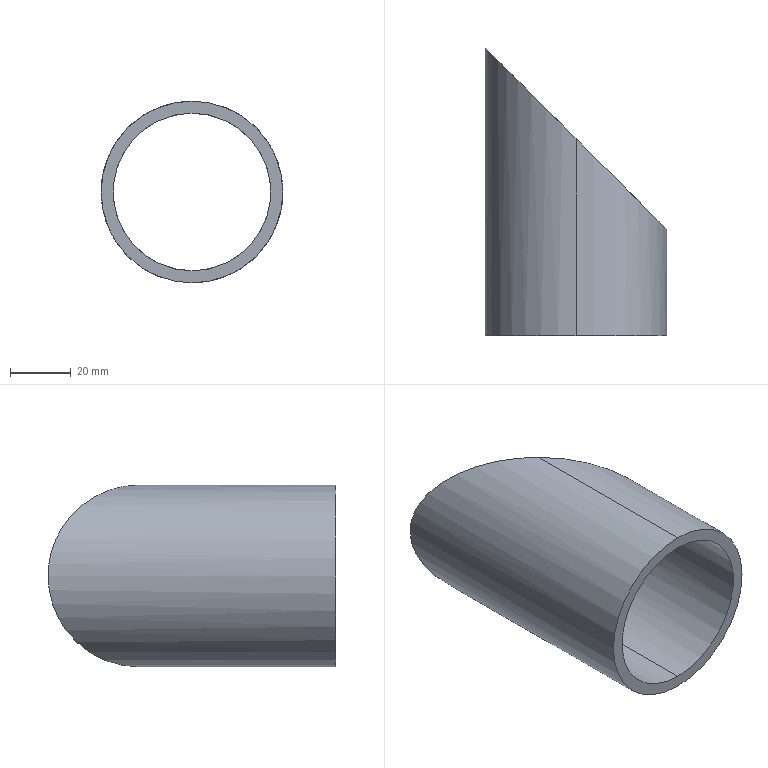Part | SolidWorks | features Extrusion 1, ICE 1 | 1 solid | 6 faces | box 60 x 95 x 60 mm | volume 45740 mm3 | cylinder 4 | plane 2 | commonest cylinder face diameters 52 x2 60 x2
STEP:
#1=CARTESIAN_POINT('',(0.,65.,-26.));
#2=VERTEX_POINT('',#1);
#3=CARTESIAN_POINT('',(0.,65.,26.));
#4=VERTEX_POINT('',#3);
#5=CARTESIAN_POINT('',(0.,65.,-26.));
#6=CARTESIAN_POINT('',(-52.,117.,-26.));
#7=CARTESIAN_POINT('',(-52.,117.,26.));
#8=CARTESIAN_POINT('',(0.,65.,26.));
#9=(BOUNDED_CURVE()B_SPLINE_CURVE(3,(#5,#6,#7,#8),.UNSPECIFIED.,.F.,.F.)B_SPLINE_CURVE_WITH_KNOTS((4,4),(1.571,4.712),.UNSPECIFIED.)CURVE()GEOMETRIC_REPRESENTATION_ITEM()RATIONAL_B_SPLINE_CURVE((1.,0.3333,0.3333,1.))REPRESENTATION_ITEM(''));
#10=EDGE_CURVE('',#2,#4,#9,.T.);
#11=ORIENTED_EDGE('',*,*,#10,.T.);
#12=CARTESIAN_POINT('',(0.,0.,26.));
#13=VERTEX_POINT('',#12);
#14=CARTESIAN_POINT('',(0.,95.,26.));
#15=DIRECTION('',(0.,-1.,0.));
#16=VECTOR('',#15,1000.);
#17=LINE('',#14,#16);
#18=EDGE_CURVE('',#4,#13,#17,.T.);
#19=ORIENTED_EDGE('',*,*,#18,.T.);
#20=CARTESIAN_POINT('',(0.,0.,-26.));
#21=VERTEX_POINT('',#20);
#22=CARTESIAN_POINT('',(0.,0.,0.));
#23=DIRECTION('',(0.,1.,0.));
#24=DIRECTION('',(0.,0.,1.));
#25=AXIS2_PLACEMENT_3D('',#22,#23,#24);
#26=CIRCLE('',#25,26.);
#27=EDGE_CURVE('',#21,#13,#26,.T.);
#28=ORIENTED_EDGE('',*,*,#27,.F.);
#29=CARTESIAN_POINT('',(0.,95.,-26.));
#30=DIRECTION('',(0.,-1.,0.));
#31=VECTOR('',#30,1000.);
#32=LINE('',#29,#31);
#33=EDGE_CURVE('',#2,#21,#32,.T.);
#34=ORIENTED_EDGE('',*,*,#33,.F.);
#35=EDGE_LOOP('',(#11,#19,#28,#34));
#36=FACE_OUTER_BOUND('',#35,.T.);
#37=CARTESIAN_POINT('',(0.,95.,0.));
#38=DIRECTION('',(0.,-1.,0.));
#39=DIRECTION('',(0.,0.,-1.));
#40=AXIS2_PLACEMENT_3D('',#37,#38,#39);
#41=CYLINDRICAL_SURFACE('',#40,26.);
#42=ADVANCED_FACE('',(#36),#41,.F.);
#43=CARTESIAN_POINT('',(0.,65.,30.));
#44=VERTEX_POINT('',#43);
#45=CARTESIAN_POINT('',(0.,65.,-30.));
#46=VERTEX_POINT('',#45);
#47=CARTESIAN_POINT('',(0.,65.,30.));
#48=CARTESIAN_POINT('',(60.,5.,30.));
#49=CARTESIAN_POINT('',(60.,5.,-30.));
#50=CARTESIAN_POINT('',(0.,65.,-30.));
#51=(BOUNDED_CURVE()B_SPLINE_CURVE(3,(#47,#48,#49,#50),.UNSPECIFIED.,.F.,.F.)B_SPLINE_CURVE_WITH_KNOTS((4,4),(4.712,7.854),.UNSPECIFIED.)CURVE()GEOMETRIC_REPRESENTATION_ITEM()RATIONAL_B_SPLINE_CURVE((1.,0.3333,0.3333,1.))REPRESENTATION_ITEM(''));
#52=EDGE_CURVE('',#44,#46,#51,.T.);
#53=ORIENTED_EDGE('',*,*,#52,.F.);
#54=CARTESIAN_POINT('',(0.,0.,30.));
#55=VERTEX_POINT('',#54);
#56=CARTESIAN_POINT('',(0.,95.,30.));
#57=DIRECTION('',(0.,-1.,0.));
#58=VECTOR('',#57,1000.);
#59=LINE('',#56,#58);
#60=EDGE_CURVE('',#44,#55,#59,.T.);
#61=ORIENTED_EDGE('',*,*,#60,.T.);
#62=CARTESIAN_POINT('',(0.,0.,-30.));
#63=VERTEX_POINT('',#62);
#64=CARTESIAN_POINT('',(0.,0.,0.));
#65=DIRECTION('',(0.,1.,0.));
#66=DIRECTION('',(0.,0.,1.));
#67=AXIS2_PLACEMENT_3D('',#64,#65,#66);
#68=CIRCLE('',#67,30.);
#69=EDGE_CURVE('',#55,#63,#68,.T.);
#70=ORIENTED_EDGE('',*,*,#69,.T.);
#71=CARTESIAN_POINT('',(0.,95.,-30.));
#72=DIRECTION('',(0.,-1.,0.));
#73=VECTOR('',#72,1000.);
#74=LINE('',#71,#73);
#75=EDGE_CURVE('',#46,#63,#74,.T.);
#76=ORIENTED_EDGE('',*,*,#75,.F.);
#77=EDGE_LOOP('',(#53,#61,#70,#76));
#78=FACE_OUTER_BOUND('',#77,.T.);
#79=CARTESIAN_POINT('',(0.,95.,0.));
#80=DIRECTION('',(0.,-1.,0.));
#81=DIRECTION('',(0.,0.,-1.));
#82=AXIS2_PLACEMENT_3D('',#79,#80,#81);
#83=CYLINDRICAL_SURFACE('',#82,30.);
#84=ADVANCED_FACE('',(#78),#83,.T.);
#85=ORIENTED_EDGE('',*,*,#60,.F.);
#86=CARTESIAN_POINT('',(0.,65.,-30.));
#87=CARTESIAN_POINT('',(-60.,125.,-30.));
#88=CARTESIAN_POINT('',(-60.,125.,30.));
#89=CARTESIAN_POINT('',(0.,65.,30.));
#90=(BOUNDED_CURVE()B_SPLINE_CURVE(3,(#86,#87,#88,#89),.UNSPECIFIED.,.F.,.F.)B_SPLINE_CURVE_WITH_KNOTS((4,4),(1.571,4.712),.UNSPECIFIED.)CURVE()GEOMETRIC_REPRESENTATION_ITEM()RATIONAL_B_SPLINE_CURVE((1.,0.3333,0.3333,1.))REPRESENTATION_ITEM(''));
#91=EDGE_CURVE('',#46,#44,#90,.T.);
#92=ORIENTED_EDGE('',*,*,#91,.F.);
#93=ORIENTED_EDGE('',*,*,#75,.T.);
#94=CARTESIAN_POINT('',(0.,0.,0.));
#95=DIRECTION('',(0.,1.,0.));
#96=DIRECTION('',(0.,0.,1.));
#97=AXIS2_PLACEMENT_3D('',#94,#95,#96);
#98=CIRCLE('',#97,30.);
#99=EDGE_CURVE('',#63,#55,#98,.T.);
#100=ORIENTED_EDGE('',*,*,#99,.T.);
#101=EDGE_LOOP('',(#85,#92,#93,#100));
#102=FACE_OUTER_BOUND('',#101,.T.);
#103=CARTESIAN_POINT('',(0.,95.,0.));
#104=DIRECTION('',(0.,-1.,0.));
#105=DIRECTION('',(0.,0.,-1.));
#106=AXIS2_PLACEMENT_3D('',#103,#104,#105);
#107=CYLINDRICAL_SURFACE('',#106,30.);
#108=ADVANCED_FACE('',(#102),#107,.T.);
#109=ORIENTED_EDGE('',*,*,#18,.F.);
#110=CARTESIAN_POINT('',(0.,65.,26.));
#111=CARTESIAN_POINT('',(52.,13.,26.));
#112=CARTESIAN_POINT('',(52.,13.,-26.));
#113=CARTESIAN_POINT('',(0.,65.,-26.));
#114=(BOUNDED_CURVE()B_SPLINE_CURVE(3,(#110,#111,#112,#113),.UNSPECIFIED.,.F.,.T.)B_SPLINE_CURVE_WITH_KNOTS((4,4),(4.712,7.854),.UNSPECIFIED.)CURVE()GEOMETRIC_REPRESENTATION_ITEM()RATIONAL_B_SPLINE_CURVE((1.,0.3333,0.3333,1.))REPRESENTATION_ITEM(''));
#115=EDGE_CURVE('',#4,#2,#114,.T.);
#116=ORIENTED_EDGE('',*,*,#115,.T.);
#117=ORIENTED_EDGE('',*,*,#33,.T.);
#118=CARTESIAN_POINT('',(0.,0.,0.));
#119=DIRECTION('',(0.,1.,0.));
#120=DIRECTION('',(0.,0.,1.));
#121=AXIS2_PLACEMENT_3D('',#118,#119,#120);
#122=CIRCLE('',#121,26.);
#123=EDGE_CURVE('',#13,#21,#122,.T.);
#124=ORIENTED_EDGE('',*,*,#123,.F.);
#125=EDGE_LOOP('',(#109,#116,#117,#124));
#126=FACE_OUTER_BOUND('',#125,.T.);
#127=CARTESIAN_POINT('',(0.,95.,0.));
#128=DIRECTION('',(0.,-1.,0.));
#129=DIRECTION('',(0.,0.,-1.));
#130=AXIS2_PLACEMENT_3D('',#127,#128,#129);
#131=CYLINDRICAL_SURFACE('',#130,26.);
#132=ADVANCED_FACE('',(#126),#131,.F.);
#133=ORIENTED_EDGE('',*,*,#99,.F.);
#134=ORIENTED_EDGE('',*,*,#69,.F.);
#135=EDGE_LOOP('',(#133,#134));
#136=FACE_OUTER_BOUND('',#135,.T.);
#137=ORIENTED_EDGE('',*,*,#27,.T.);
#138=ORIENTED_EDGE('',*,*,#123,.T.);
#139=EDGE_LOOP('',(#137,#138));
#140=FACE_BOUND('',#139,.T.);
#141=CARTESIAN_POINT('',(0.,0.,0.));
#142=DIRECTION('',(0.,1.,0.));
#143=DIRECTION('',(0.,0.,1.));
#144=AXIS2_PLACEMENT_3D('',#141,#142,#143);
#145=PLANE('',#144);
#146=ADVANCED_FACE('',(#136,#140),#145,.F.);
#147=ORIENTED_EDGE('',*,*,#10,.F.);
#148=ORIENTED_EDGE('',*,*,#115,.F.);
#149=EDGE_LOOP('',(#147,#148));
#150=FACE_BOUND('',#149,.T.);
#151=ORIENTED_EDGE('',*,*,#91,.T.);
#152=ORIENTED_EDGE('',*,*,#52,.T.);
#153=EDGE_LOOP('',(#151,#152));
#154=FACE_OUTER_BOUND('',#153,.T.);
#155=CARTESIAN_POINT('',(-30.,95.,196.722));
#156=DIRECTION('',(0.7071,0.7071,0.));
#157=DIRECTION('',(-0.7071,0.7071,0.));
#158=AXIS2_PLACEMENT_3D('',#155,#156,#157);
#159=PLANE('',#158);
#160=ADVANCED_FACE('',(#150,#154),#159,.T.);
#161=CLOSED_SHELL('',(#42,#84,#108,#132,#146,#160));
#162=MANIFOLD_SOLID_BREP('',#161);
#163=CARTESIAN_POINT('',(0.,0.,0.));
#164=DIRECTION('',(0.,0.,1.));
#165=DIRECTION('',(1.,0.,0.));
#166=AXIS2_PLACEMENT_3D('',#163,#164,#165);
#167=(LENGTH_UNIT()NAMED_UNIT(*)SI_UNIT(.MILLI.,.METRE.));
#168=UNCERTAINTY_MEASURE_WITH_UNIT(LENGTH_MEASURE(0.00001),#167,'','');
#169=(NAMED_UNIT(*)PLANE_ANGLE_UNIT()SI_UNIT($,.RADIAN.));
#170=(NAMED_UNIT(*)SI_UNIT($,.STERADIAN.)SOLID_ANGLE_UNIT());
#171=(GEOMETRIC_REPRESENTATION_CONTEXT(3)GLOBAL_UNCERTAINTY_ASSIGNED_CONTEXT((#168))GLOBAL_UNIT_ASSIGNED_CONTEXT((#167,#169,#170))REPRESENTATION_CONTEXT('',''));
#172=ADVANCED_BREP_SHAPE_REPRESENTATION('',(#162,#166),#171);